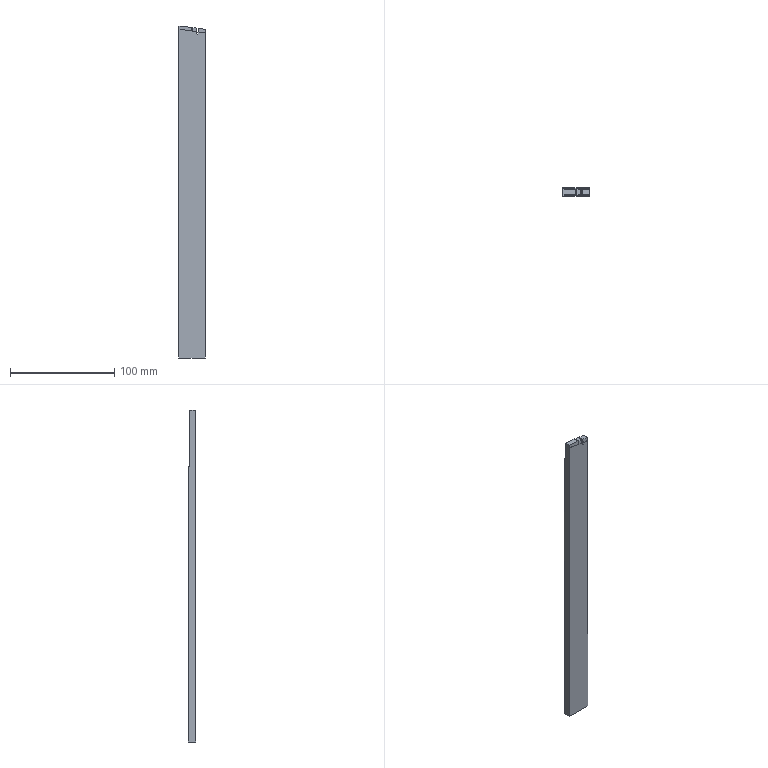Part | STEP file | P011002L006-000 | 1 solid | 92 faces | box 25 x 8.891 x 318.622 mm | volume 57302 mm3 | plane 49 | spline 17 | cone 10 | other 10 | cylinder 6 | commonest cylinder face diameters 4.167 x2 4.983 x2 5 x2